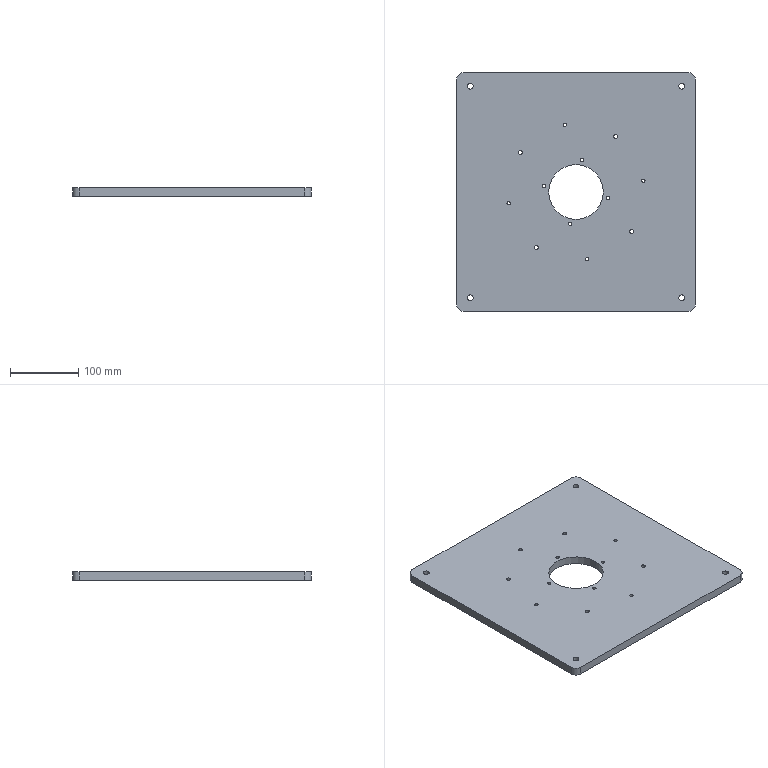Part | STEP file | 11-FG-Z00111 | 1 solid | 56 faces | box 350 x 350 x 12 mm | volume 1399212 mm3 | cylinder 46 | plane 10 | commonest cylinder face diameters 5 x16 6 x8 8.5 x8 25 x8 20 x4 80 x2